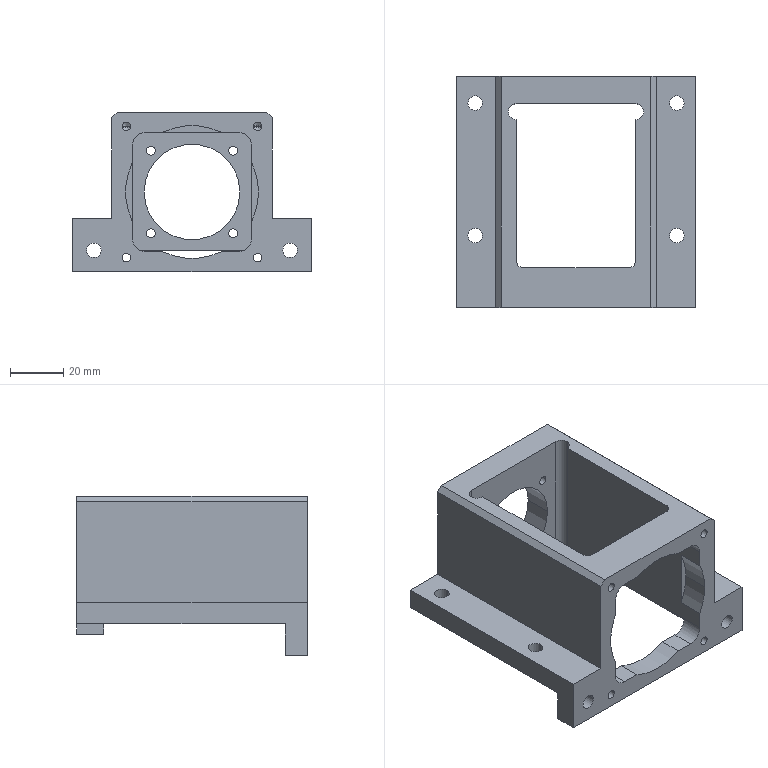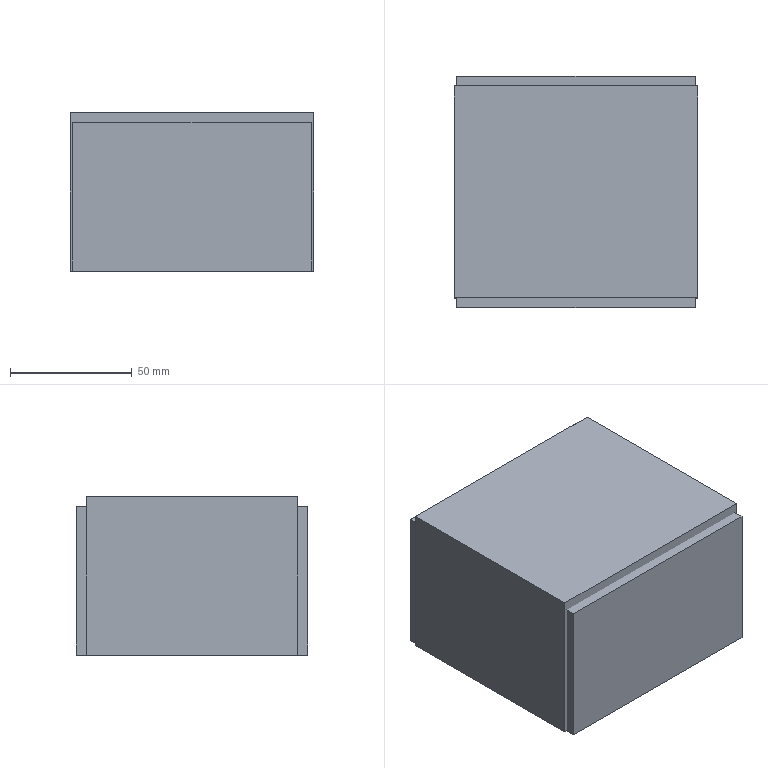CAM job | NX | 3-axis milling, drilling | part box 90 x 87.1 x 60 mm | stock box 100 x 95.1 x 65 mm
Tools:
number,name,description,diameter,corner_radius,flute_length,length,flutes
1,D63,Milling Tool-5 Parameters,63.0,0.0,50.0,75.0,2
20,D20,Milling Tool-5 Parameters,20.0,0.0,50.0,75.0,2
7,D6A45,Milling Tool-5 Parameters,6.0,0.0,3.0,3.0,2
16,6.0ZT,Drilling Tool,6.0,0.0,35.0,50.0,2
11,D10JING,Milling Tool-5 Parameters,10.0,0.0,50.0,75.0,2
4,D4,Milling Tool-5 Parameters,4.0,0.0,50.0,75.0,2
10,D10,Milling Tool-5 Parameters,10.0,0.0,50.0,75.0,2
6,D6,Milling Tool-5 Parameters,6.0,0.0,50.0,75.0,2
15,5.5ZT,Drilling Tool,5.5,0.0,35.0,50.0,2
Operations:
program,operation,operation_type,tool,method,geometry_group,spindle_rpm,surface_speed,feed_per_tooth,feed_cut,feed_plunge,cut_length_mm,path_length_mm,cut_time_min,machine_time_min
1-93-90-65毛胚,FLOOR_WALL,VolumeBased25DMillingOperation,D63,METHOD,A,6500.0,1286.0,0.0962,1250.0,100.0,564.897,618.897,0.4519,0.4573
1-93-90-65毛胚,DRILLING_COPY_1,Operation,D6A45,METHOD,A,3000.0,56.0,0.0333,200.0,0.0,9.2,126.5,0.046,0.0577
1-93-90-65毛胚,DRILLING_COPY_1_COPY,Operation,6.0ZT,METHOD,A,2000.0,15.0,0.0375,150.0,0.0,108.605,325.31,0.724,0.7457
1-93-90-65毛胚,CAVITY_MILL,CavityMilling,D20,METHOD,A,7000.0,439.0,0.1571,2200.0,1000.0,71225.803,79293.752,34.912,35.907
1-93-90-65毛胚,ZLEVEL_PROFILE_COPY_COPY_1_1_COPY_COPY,ZLevelMilling,D20,METHOD,A,7000.0,439.0,0.0571,800.0,100.0,481.101,664.038,0.6014,0.6197
1-93-90-65毛胚,ZLEVEL_PROFILE_COPY_COPY_1_1_COPY_COPY_COPY,ZLevelMilling,D20,METHOD,A,7000.0,439.0,0.0571,800.0,100.0,768.302,908.729,0.9604,0.9744
1-93-90-65毛胚,ZLEVEL_PROFILE_COPY_COPY_1_1_COPY_COPY_COPY_COPY,ZLevelMilling,D20,METHOD,A,7000.0,439.0,0.0571,800.0,100.0,443.151,621.151,0.5539,0.5717
1-93-90-65毛胚,ZLEVEL_PROFILE_COPY_1,ZLevelMilling,D10JING,METHOD,A,7000.0,87.0,0.1071,1500.0,1000.0,7543.58,11352.552,5.474,5.855
1-93-90-65毛胚,ZLEVEL_PROFILE_COPY_1_1_COPY,ZLevelMilling,D6,METHOD,A,4000.0,75.0,0.0625,500.0,1000.0,3977.336,5198.533,7.436,7.559
1-93-90-65毛胚,ZLEVEL_PROFILE_COPY_1_1,ZLevelMilling,D4,METHOD,A,7000.0,87.0,0.1071,1500.0,1000.0,415.741,803.196,0.2957,0.3344
1-93-90-65毛胚,ZLEVEL_PROFILE_COPY_1_COPY_COPY_COPY_COPY_2_COPY,ZLevelMilling,D6A45,METHOD,A,7000.0,131.0,0.0714,1000.0,1000.0,511.877,713.776,0.5119,0.5321
1-93-90-65毛胚,ZLEVEL_PROFILE_COPY_1_COPY_COPY_COPY_COPY_2_COPY_COPY,ZLevelMilling,D6A45,METHOD,A,7000.0,131.0,0.0714,1000.0,1000.0,290.654,1414.99,0.2907,0.4031
2-93-90-65毛胚,FLOOR_WALL_COPY,VolumeBased25DMillingOperation,D63,METHOD,B,6500.0,1286.0,0.0962,1250.0,100.0,2785.485,3748.652,2.228,2.325
2-93-90-65毛胚,ADAPTIVE_MILLING,CavityMilling,D10,METHOD,B,7000.0,219.0,0.2143,3000.0,1000.0,13947.938,14873.895,4.661,4.754
2-93-90-65毛胚,DRILLING_COPY_1_1,Operation,D6A45,METHOD,B,3000.0,56.0,0.0333,200.0,0.0,20.4,325.002,0.102,0.1325
2-93-90-65毛胚,DRILLING_COPY_1_COPY_COPY_1_COPY_1,Operation,5.5ZT,METHOD,B,2000.0,41.0,0.075,300.0,0.0,56.609,382.458,0.1887,0.2213
2-93-90-65毛胚,FLOOR_WALL_1_COPY_1,VolumeBased25DMillingOperation,D10JING,METHOD,B,7000.0,87.0,0.0714,1000.0,100.0,1550.955,2104.942,1.551,1.618
2-93-90-65毛胚,ZLEVEL_PROFILE_COPY_COPY_1_1_COPY_COPY_COPY_COPY_COPY,ZLevelMilling,D10JING,METHOD,B,7000.0,439.0,0.0571,800.0,100.0,114.348,196.348,0.1429,0.1511
2-93-90-65毛胚,ZLEVEL_PROFILE_COPY_1_COPY_COPY_COPY_COPY_2_COPY_COPY_1,ZLevelMilling,D6A45,METHOD,B,7000.0,131.0,0.0714,1000.0,1000.0,205.722,267.722,0.2057,0.2119
2-93-90-65毛胚,ZLEVEL_PROFILE_COPY_1_COPY_COPY_COPY_COPY_2_COPY_COPY_1_COPY,ZLevelMilling,D6A45,METHOD,B,7000.0,131.0,0.0714,1000.0,1000.0,119.722,197.722,0.1197,0.1275
2-93-90-65毛胚,ZLEVEL_PROFILE_COPY_1_COPY_COPY_COPY_COPY_2_COPY_COPY_1_COPY_COPY,ZLevelMilling,D6A45,METHOD,B,7000.0,131.0,0.0714,1000.0,1000.0,395.972,1505.375,0.396,0.5069